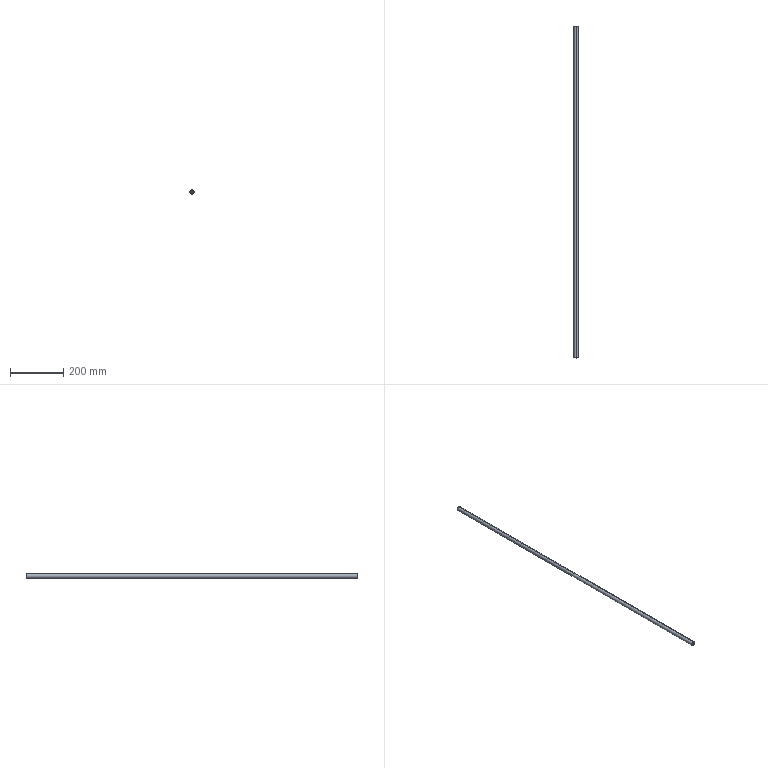Part | STEP file | PN_0027 | 1 solid | 16 faces | box 16 x 1252 x 16 mm | volume 251030 mm3 | cone 8 | cylinder 6 | plane 2 | commonest cylinder face diameters 5 x4 16 x2
STEP:
#1=CARTESIAN_POINT('',(0.,0.,0.));
#2=DIRECTION('',(0.,0.,1.));
#3=DIRECTION('',(1.,0.,0.));
#4=AXIS2_PLACEMENT_3D('',#1,#2,#3);
#5=CARTESIAN_POINT('',(0.,1252.,7.5));
#6=VERTEX_POINT('',#5);
#7=CARTESIAN_POINT('',(0.,1252.,-7.5));
#8=VERTEX_POINT('',#7);
#9=CARTESIAN_POINT('',(0.,1252.,0.));
#10=DIRECTION('',(0.,1.,0.));
#11=DIRECTION('',(0.,0.,1.));
#12=AXIS2_PLACEMENT_3D('',#9,#10,#11);
#13=CIRCLE('',#12,7.5);
#14=CARTESIAN_POINT('',(0.,1252.,0.));
#15=DIRECTION('',(0.,-1.,0.));
#16=DIRECTION('',(0.,0.,-1.));
#17=AXIS2_PLACEMENT_3D('',#14,#15,#16);
#18=CONICAL_SURFACE('',#17,7.5,0.7854);
#19=CARTESIAN_POINT('',(3.142,0.));
#20=DIRECTION('',(-1.,0.));
#21=VECTOR('',#20,1.);
#22=LINE('',#19,#21);
#23=(GEOMETRIC_REPRESENTATION_CONTEXT(2)PARAMETRIC_REPRESENTATION_CONTEXT()REPRESENTATION_CONTEXT('',''));
#24=DEFINITIONAL_REPRESENTATION('',(#22),#23);
#25=PCURVE('',#18,#24);
#26=CARTESIAN_POINT('',(0.,1252.,0.));
#27=DIRECTION('',(0.,1.,0.));
#28=DIRECTION('',(0.,0.,1.));
#29=AXIS2_PLACEMENT_3D('',#26,#27,#28);
#30=PLANE('',#29);
#31=CARTESIAN_POINT('',(0.,0.));
#32=DIRECTION('',(1.,0.));
#33=AXIS2_PLACEMENT_2D('',#31,#32);
#34=CIRCLE('',#33,7.5);
#35=(GEOMETRIC_REPRESENTATION_CONTEXT(2)PARAMETRIC_REPRESENTATION_CONTEXT()REPRESENTATION_CONTEXT('',''));
#36=DEFINITIONAL_REPRESENTATION('',(#34),#35);
#37=PCURVE('',#30,#36);
#38=SURFACE_CURVE('',#13,(#25,#37),.PCURVE_S1.);
#39=EDGE_CURVE('',#6,#8,#38,.T.);
#40=ORIENTED_EDGE('',*,*,#39,.F.);
#41=CARTESIAN_POINT('',(0.,1251.5,8.));
#42=VERTEX_POINT('',#41);
#43=CARTESIAN_POINT('',(0.,1252.,7.5));
#44=DIRECTION('',(0.,-0.7071,0.7071));
#45=VECTOR('',#44,1.);
#46=LINE('',#43,#45);
#47=CARTESIAN_POINT('',(3.142,0.));
#48=DIRECTION('',(0.,1.));
#49=VECTOR('',#48,1.);
#50=LINE('',#47,#49);
#51=(GEOMETRIC_REPRESENTATION_CONTEXT(2)PARAMETRIC_REPRESENTATION_CONTEXT()REPRESENTATION_CONTEXT('',''));
#52=DEFINITIONAL_REPRESENTATION('',(#50),#51);
#53=PCURVE('',#18,#52);
#54=CARTESIAN_POINT('',(0.,1252.,0.));
#55=DIRECTION('',(0.,-1.,0.));
#56=DIRECTION('',(0.,0.,-1.));
#57=AXIS2_PLACEMENT_3D('',#54,#55,#56);
#58=CONICAL_SURFACE('',#57,7.5,0.7854);
#59=CARTESIAN_POINT('',(3.142,0.));
#60=DIRECTION('',(0.,1.));
#61=VECTOR('',#60,1.);
#62=LINE('',#59,#61);
#63=(GEOMETRIC_REPRESENTATION_CONTEXT(2)PARAMETRIC_REPRESENTATION_CONTEXT()REPRESENTATION_CONTEXT('',''));
#64=DEFINITIONAL_REPRESENTATION('',(#62),#63);
#65=PCURVE('',#58,#64);
#66=SURFACE_CURVE('',#46,(#53,#65),.PCURVE_S1.);
#67=EDGE_CURVE('',#6,#42,#66,.T.);
#68=ORIENTED_EDGE('',*,*,#67,.T.);
#69=CARTESIAN_POINT('',(0.,1251.5,-8.));
#70=VERTEX_POINT('',#69);
#71=CARTESIAN_POINT('',(0.,1251.5,0.));
#72=DIRECTION('',(0.,-1.,0.));
#73=DIRECTION('',(0.,0.,1.));
#74=AXIS2_PLACEMENT_3D('',#71,#72,#73);
#75=CIRCLE('',#74,8.);
#76=CARTESIAN_POINT('',(-3.142,0.5));
#77=DIRECTION('',(1.,0.));
#78=VECTOR('',#77,1.);
#79=LINE('',#76,#78);
#80=(GEOMETRIC_REPRESENTATION_CONTEXT(2)PARAMETRIC_REPRESENTATION_CONTEXT()REPRESENTATION_CONTEXT('',''));
#81=DEFINITIONAL_REPRESENTATION('',(#79),#80);
#82=PCURVE('',#18,#81);
#83=CARTESIAN_POINT('',(0.,1252.,0.));
#84=DIRECTION('',(0.,-1.,0.));
#85=DIRECTION('',(0.,0.,-1.));
#86=AXIS2_PLACEMENT_3D('',#83,#84,#85);
#87=CYLINDRICAL_SURFACE('',#86,8.);
#88=CARTESIAN_POINT('',(-3.142,0.5));
#89=DIRECTION('',(1.,0.));
#90=VECTOR('',#89,1.);
#91=LINE('',#88,#90);
#92=(GEOMETRIC_REPRESENTATION_CONTEXT(2)PARAMETRIC_REPRESENTATION_CONTEXT()REPRESENTATION_CONTEXT('',''));
#93=DEFINITIONAL_REPRESENTATION('',(#91),#92);
#94=PCURVE('',#87,#93);
#95=SURFACE_CURVE('',#75,(#82,#94),.PCURVE_S1.);
#96=EDGE_CURVE('',#70,#42,#95,.T.);
#97=ORIENTED_EDGE('',*,*,#96,.F.);
#98=CARTESIAN_POINT('',(0.,1252.,-7.5));
#99=DIRECTION('',(0.,-0.7071,-0.7071));
#100=VECTOR('',#99,1.);
#101=LINE('',#98,#100);
#102=CARTESIAN_POINT('',(0.,0.));
#103=DIRECTION('',(0.,1.));
#104=VECTOR('',#103,1.);
#105=LINE('',#102,#104);
#106=(GEOMETRIC_REPRESENTATION_CONTEXT(2)PARAMETRIC_REPRESENTATION_CONTEXT()REPRESENTATION_CONTEXT('',''));
#107=DEFINITIONAL_REPRESENTATION('',(#105),#106);
#108=PCURVE('',#18,#107);
#109=CARTESIAN_POINT('',(6.283,0.));
#110=DIRECTION('',(0.,1.));
#111=VECTOR('',#110,1.);
#112=LINE('',#109,#111);
#113=(GEOMETRIC_REPRESENTATION_CONTEXT(2)PARAMETRIC_REPRESENTATION_CONTEXT()REPRESENTATION_CONTEXT('',''));
#114=DEFINITIONAL_REPRESENTATION('',(#112),#113);
#115=PCURVE('',#58,#114);
#116=SURFACE_CURVE('',#101,(#108,#115),.PCURVE_S1.);
#117=EDGE_CURVE('',#8,#70,#116,.T.);
#118=ORIENTED_EDGE('',*,*,#117,.F.);
#119=EDGE_LOOP('',(#40,#68,#97,#118));
#120=FACE_BOUND('',#119,.T.);
#121=ADVANCED_FACE('',(#120),#18,.T.);
#122=CARTESIAN_POINT('',(0.,0.,-7.5));
#123=VERTEX_POINT('',#122);
#124=CARTESIAN_POINT('',(0.,0.,7.5));
#125=VERTEX_POINT('',#124);
#126=CARTESIAN_POINT('',(0.,0.,0.));
#127=DIRECTION('',(0.,-1.,0.));
#128=DIRECTION('',(0.,0.,1.));
#129=AXIS2_PLACEMENT_3D('',#126,#127,#128);
#130=CIRCLE('',#129,7.5);
#131=CARTESIAN_POINT('',(0.,0.5,0.));
#132=DIRECTION('',(0.,1.,0.));
#133=DIRECTION('',(0.,0.,1.));
#134=AXIS2_PLACEMENT_3D('',#131,#132,#133);
#135=CONICAL_SURFACE('',#134,8.,0.7854);
#136=CARTESIAN_POINT('',(6.283,-0.5));
#137=DIRECTION('',(-1.,0.));
#138=VECTOR('',#137,1.);
#139=LINE('',#136,#138);
#140=(GEOMETRIC_REPRESENTATION_CONTEXT(2)PARAMETRIC_REPRESENTATION_CONTEXT()REPRESENTATION_CONTEXT('',''));
#141=DEFINITIONAL_REPRESENTATION('',(#139),#140);
#142=PCURVE('',#135,#141);
#143=CARTESIAN_POINT('',(0.,0.,0.));
#144=DIRECTION('',(0.,1.,0.));
#145=DIRECTION('',(0.,0.,1.));
#146=AXIS2_PLACEMENT_3D('',#143,#144,#145);
#147=PLANE('',#146);
#148=CARTESIAN_POINT('',(7.5,0.));
#149=CARTESIAN_POINT('',(7.5,-12.99));
#150=CARTESIAN_POINT('',(-3.75,-6.495));
#151=CARTESIAN_POINT('',(-15.,0.));
#152=CARTESIAN_POINT('',(-3.75,6.495));
#153=CARTESIAN_POINT('',(7.5,12.99));
#154=CARTESIAN_POINT('',(7.5,0.));
#155=(BOUNDED_CURVE()B_SPLINE_CURVE(2,(#148,#149,#150,#151,#152,#153,#154),.UNSPECIFIED.,.T.,.F.)B_SPLINE_CURVE_WITH_KNOTS((1,2,2,2,2,1),(-2.094,0.,2.094,4.189,6.283,8.378),.UNSPECIFIED.)CURVE()GEOMETRIC_REPRESENTATION_ITEM()RATIONAL_B_SPLINE_CURVE((1.,0.5,1.,0.5,1.,0.5,1.))REPRESENTATION_ITEM(''));
#156=(GEOMETRIC_REPRESENTATION_CONTEXT(2)PARAMETRIC_REPRESENTATION_CONTEXT()REPRESENTATION_CONTEXT('',''));
#157=DEFINITIONAL_REPRESENTATION('',(#155),#156);
#158=PCURVE('',#147,#157);
#159=SURFACE_CURVE('',#130,(#142,#158),.PCURVE_S1.);
#160=EDGE_CURVE('',#123,#125,#159,.T.);
#161=ORIENTED_EDGE('',*,*,#160,.F.);
#162=CARTESIAN_POINT('',(0.,0.5,-8.));
#163=VERTEX_POINT('',#162);
#164=CARTESIAN_POINT('',(0.,0.5,-8.));
#165=DIRECTION('',(0.,0.7071,-0.7071));
#166=VECTOR('',#165,1.);
#167=LINE('',#164,#166);
#168=CARTESIAN_POINT('',(3.142,0.));
#169=DIRECTION('',(0.,1.));
#170=VECTOR('',#169,1.);
#171=LINE('',#168,#170);
#172=(GEOMETRIC_REPRESENTATION_CONTEXT(2)PARAMETRIC_REPRESENTATION_CONTEXT()REPRESENTATION_CONTEXT('',''));
#173=DEFINITIONAL_REPRESENTATION('',(#171),#172);
#174=PCURVE('',#135,#173);
#175=CARTESIAN_POINT('',(0.,0.5,0.));
#176=DIRECTION('',(0.,1.,0.));
#177=DIRECTION('',(0.,0.,1.));
#178=AXIS2_PLACEMENT_3D('',#175,#176,#177);
#179=CONICAL_SURFACE('',#178,8.,0.7854);
#180=CARTESIAN_POINT('',(3.142,0.));
#181=DIRECTION('',(0.,1.));
#182=VECTOR('',#181,1.);
#183=LINE('',#180,#182);
#184=(GEOMETRIC_REPRESENTATION_CONTEXT(2)PARAMETRIC_REPRESENTATION_CONTEXT()REPRESENTATION_CONTEXT('',''));
#185=DEFINITIONAL_REPRESENTATION('',(#183),#184);
#186=PCURVE('',#179,#185);
#187=SURFACE_CURVE('',#167,(#174,#186),.PCURVE_S1.);
#188=EDGE_CURVE('',#123,#163,#187,.T.);
#189=ORIENTED_EDGE('',*,*,#188,.T.);
#190=CARTESIAN_POINT('',(0.,0.5,8.));
#191=VERTEX_POINT('',#190);
#192=CARTESIAN_POINT('',(0.,0.5,0.));
#193=DIRECTION('',(0.,1.,0.));
#194=DIRECTION('',(0.,0.,1.));
#195=AXIS2_PLACEMENT_3D('',#192,#193,#194);
#196=CIRCLE('',#195,8.);
#197=CARTESIAN_POINT('',(0.,0.));
#198=DIRECTION('',(1.,0.));
#199=VECTOR('',#198,1.);
#200=LINE('',#197,#199);
#201=(GEOMETRIC_REPRESENTATION_CONTEXT(2)PARAMETRIC_REPRESENTATION_CONTEXT()REPRESENTATION_CONTEXT('',''));
#202=DEFINITIONAL_REPRESENTATION('',(#200),#201);
#203=PCURVE('',#135,#202);
#204=CARTESIAN_POINT('',(3.142,1251.5));
#205=DIRECTION('',(-1.,0.));
#206=VECTOR('',#205,1.);
#207=LINE('',#204,#206);
#208=(GEOMETRIC_REPRESENTATION_CONTEXT(2)PARAMETRIC_REPRESENTATION_CONTEXT()REPRESENTATION_CONTEXT('',''));
#209=DEFINITIONAL_REPRESENTATION('',(#207),#208);
#210=PCURVE('',#87,#209);
#211=SURFACE_CURVE('',#196,(#203,#210),.PCURVE_S1.);
#212=EDGE_CURVE('',#191,#163,#211,.T.);
#213=ORIENTED_EDGE('',*,*,#212,.F.);
#214=CARTESIAN_POINT('',(0.,0.5,8.));
#215=DIRECTION('',(0.,0.7071,0.7071));
#216=VECTOR('',#215,1.);
#217=LINE('',#214,#216);
#218=CARTESIAN_POINT('',(0.,0.));
#219=DIRECTION('',(0.,1.));
#220=VECTOR('',#219,1.);
#221=LINE('',#218,#220);
#222=(GEOMETRIC_REPRESENTATION_CONTEXT(2)PARAMETRIC_REPRESENTATION_CONTEXT()REPRESENTATION_CONTEXT('',''));
#223=DEFINITIONAL_REPRESENTATION('',(#221),#222);
#224=PCURVE('',#135,#223);
#225=CARTESIAN_POINT('',(6.283,0.));
#226=DIRECTION('',(0.,1.));
#227=VECTOR('',#226,1.);
#228=LINE('',#225,#227);
#229=(GEOMETRIC_REPRESENTATION_CONTEXT(2)PARAMETRIC_REPRESENTATION_CONTEXT()REPRESENTATION_CONTEXT('',''));
#230=DEFINITIONAL_REPRESENTATION('',(#228),#229);
#231=PCURVE('',#179,#230);
#232=SURFACE_CURVE('',#217,(#224,#231),.PCURVE_S1.);
#233=EDGE_CURVE('',#125,#191,#232,.T.);
#234=ORIENTED_EDGE('',*,*,#233,.F.);
#235=EDGE_LOOP('',(#161,#189,#213,#234));
#236=FACE_BOUND('',#235,.T.);
#237=ADVANCED_FACE('',(#236),#135,.T.);
#238=CARTESIAN_POINT('',(0.,17.,-2.5));
#239=VERTEX_POINT('',#238);
#240=CARTESIAN_POINT('',(0.,0.,-2.5));
#241=VERTEX_POINT('',#240);
#242=CARTESIAN_POINT('',(0.,0.,-2.5));
#243=DIRECTION('',(0.,-1.,0.));
#244=VECTOR('',#243,1.);
#245=LINE('',#242,#244);
#246=CARTESIAN_POINT('',(0.,0.,0.));
#247=DIRECTION('',(0.,-1.,0.));
#248=DIRECTION('',(0.,0.,-1.));
#249=AXIS2_PLACEMENT_3D('',#246,#247,#248);
#250=CYLINDRICAL_SURFACE('',#249,2.5);
#251=CARTESIAN_POINT('',(6.283,0.));
#252=DIRECTION('',(0.,1.));
#253=VECTOR('',#252,1.);
#254=LINE('',#251,#253);
#255=(GEOMETRIC_REPRESENTATION_CONTEXT(2)PARAMETRIC_REPRESENTATION_CONTEXT()REPRESENTATION_CONTEXT('',''));
#256=DEFINITIONAL_REPRESENTATION('',(#254),#255);
#257=PCURVE('',#250,#256);
#258=CARTESIAN_POINT('',(0.,0.,0.));
#259=DIRECTION('',(0.,-1.,0.));
#260=DIRECTION('',(0.,0.,-1.));
#261=AXIS2_PLACEMENT_3D('',#258,#259,#260);
#262=CYLINDRICAL_SURFACE('',#261,2.5);
#263=CARTESIAN_POINT('',(0.,0.));
#264=DIRECTION('',(0.,1.));
#265=VECTOR('',#264,1.);
#266=LINE('',#263,#265);
#267=(GEOMETRIC_REPRESENTATION_CONTEXT(2)PARAMETRIC_REPRESENTATION_CONTEXT()REPRESENTATION_CONTEXT('',''));
#268=DEFINITIONAL_REPRESENTATION('',(#266),#267);
#269=PCURVE('',#262,#268);
#270=SURFACE_CURVE('',#245,(#257,#269),.PCURVE_S1.);
#271=EDGE_CURVE('',#239,#241,#270,.T.);
#272=ORIENTED_EDGE('',*,*,#271,.T.);
#273=CARTESIAN_POINT('',(0.,0.,2.5));
#274=VERTEX_POINT('',#273);
#275=CARTESIAN_POINT('',(0.,0.,0.));
#276=DIRECTION('',(0.,-1.,0.));
#277=DIRECTION('',(0.,0.,-1.));
#278=AXIS2_PLACEMENT_3D('',#275,#276,#277);
#279=CIRCLE('',#278,2.5);
#280=CARTESIAN_POINT('',(0.,0.));
#281=DIRECTION('',(1.,0.));
#282=VECTOR('',#281,1.);
#283=LINE('',#280,#282);
#284=(GEOMETRIC_REPRESENTATION_CONTEXT(2)PARAMETRIC_REPRESENTATION_CONTEXT()REPRESENTATION_CONTEXT('',''));
#285=DEFINITIONAL_REPRESENTATION('',(#283),#284);
#286=PCURVE('',#250,#285);
#287=CARTESIAN_POINT('',(-2.5,0.));
#288=CARTESIAN_POINT('',(-2.5,4.33));
#289=CARTESIAN_POINT('',(1.25,2.165));
#290=CARTESIAN_POINT('',(5.,0.));
#291=CARTESIAN_POINT('',(1.25,-2.165));
#292=CARTESIAN_POINT('',(-2.5,-4.33));
#293=CARTESIAN_POINT('',(-2.5,0.));
#294=(BOUNDED_CURVE()B_SPLINE_CURVE(2,(#287,#288,#289,#290,#291,#292,#293),.UNSPECIFIED.,.T.,.F.)B_SPLINE_CURVE_WITH_KNOTS((1,2,2,2,2,1),(-2.094,0.,2.094,4.189,6.283,8.378),.UNSPECIFIED.)CURVE()GEOMETRIC_REPRESENTATION_ITEM()RATIONAL_B_SPLINE_CURVE((1.,0.5,1.,0.5,1.,0.5,1.))REPRESENTATION_ITEM(''));
#295=(GEOMETRIC_REPRESENTATION_CONTEXT(2)PARAMETRIC_REPRESENTATION_CONTEXT()REPRESENTATION_CONTEXT('',''));
#296=DEFINITIONAL_REPRESENTATION('',(#294),#295);
#297=PCURVE('',#147,#296);
#298=SURFACE_CURVE('',#279,(#286,#297),.PCURVE_S1.);
#299=EDGE_CURVE('',#274,#241,#298,.T.);
#300=ORIENTED_EDGE('',*,*,#299,.F.);
#301=CARTESIAN_POINT('',(0.,17.,2.5));
#302=VERTEX_POINT('',#301);
#303=CARTESIAN_POINT('',(0.,0.,2.5));
#304=DIRECTION('',(0.,-1.,0.));
#305=VECTOR('',#304,1.);
#306=LINE('',#303,#305);
#307=CARTESIAN_POINT('',(3.142,0.));
#308=DIRECTION('',(0.,1.));
#309=VECTOR('',#308,1.);
#310=LINE('',#307,#309);
#311=(GEOMETRIC_REPRESENTATION_CONTEXT(2)PARAMETRIC_REPRESENTATION_CONTEXT()REPRESENTATION_CONTEXT('',''));
#312=DEFINITIONAL_REPRESENTATION('',(#310),#311);
#313=PCURVE('',#250,#312);
#314=CARTESIAN_POINT('',(3.142,0.));
#315=DIRECTION('',(0.,1.));
#316=VECTOR('',#315,1.);
#317=LINE('',#314,#316);
#318=(GEOMETRIC_REPRESENTATION_CONTEXT(2)PARAMETRIC_REPRESENTATION_CONTEXT()REPRESENTATION_CONTEXT('',''));
#319=DEFINITIONAL_REPRESENTATION('',(#317),#318);
#320=PCURVE('',#262,#319);
#321=SURFACE_CURVE('',#306,(#313,#320),.PCURVE_S1.);
#322=EDGE_CURVE('',#302,#274,#321,.T.);
#323=ORIENTED_EDGE('',*,*,#322,.F.);
#324=CARTESIAN_POINT('',(0.,17.,0.));
#325=DIRECTION('',(0.,-1.,0.));
#326=DIRECTION('',(0.,0.,-1.));
#327=AXIS2_PLACEMENT_3D('',#324,#325,#326);
#328=CIRCLE('',#327,2.5);
#329=CARTESIAN_POINT('',(0.,-17.));
#330=DIRECTION('',(1.,0.));
#331=VECTOR('',#330,1.);
#332=LINE('',#329,#331);
#333=(GEOMETRIC_REPRESENTATION_CONTEXT(2)PARAMETRIC_REPRESENTATION_CONTEXT()REPRESENTATION_CONTEXT('',''));
#334=DEFINITIONAL_REPRESENTATION('',(#332),#333);
#335=PCURVE('',#250,#334);
#336=CARTESIAN_POINT('',(0.,17.,0.));
#337=DIRECTION('',(0.,-1.,0.));
#338=DIRECTION('',(0.,0.,-1.));
#339=AXIS2_PLACEMENT_3D('',#336,#337,#338);
#340=CONICAL_SURFACE('',#339,2.5,1.03);
#341=CARTESIAN_POINT('',(0.,0.));
#342=DIRECTION('',(1.,0.));
#343=VECTOR('',#342,1.);
#344=LINE('',#341,#343);
#345=(GEOMETRIC_REPRESENTATION_CONTEXT(2)PARAMETRIC_REPRESENTATION_CONTEXT()REPRESENTATION_CONTEXT('',''));
#346=DEFINITIONAL_REPRESENTATION('',(#344),#345);
#347=PCURVE('',#340,#346);
#348=SURFACE_CURVE('',#328,(#335,#347),.PCURVE_S1.);
#349=EDGE_CURVE('',#302,#239,#348,.T.);
#350=ORIENTED_EDGE('',*,*,#349,.T.);
#351=EDGE_LOOP('',(#272,#300,#323,#350));
#352=FACE_BOUND('',#351,.F.);
#353=ADVANCED_FACE('',(#352),#250,.F.);
#354=ORIENTED_EDGE('',*,*,#349,.F.);
#355=CARTESIAN_POINT('',(0.,18.502,0.));
#356=VERTEX_POINT('',#355);
#357=CARTESIAN_POINT('',(0.,17.,2.5));
#358=DIRECTION('',(0.,-0.515,0.8572));
#359=VECTOR('',#358,1.);
#360=LINE('',#357,#359);
#361=CARTESIAN_POINT('',(3.142,0.));
#362=DIRECTION('',(0.,1.));
#363=VECTOR('',#362,1.);
#364=LINE('',#361,#363);
#365=(GEOMETRIC_REPRESENTATION_CONTEXT(2)PARAMETRIC_REPRESENTATION_CONTEXT()REPRESENTATION_CONTEXT('',''));
#366=DEFINITIONAL_REPRESENTATION('',(#364),#365);
#367=PCURVE('',#340,#366);
#368=CARTESIAN_POINT('',(0.,17.,0.));
#369=DIRECTION('',(0.,-1.,0.));
#370=DIRECTION('',(0.,0.,-1.));
#371=AXIS2_PLACEMENT_3D('',#368,#369,#370);
#372=CONICAL_SURFACE('',#371,2.5,1.03);
#373=CARTESIAN_POINT('',(3.142,0.));
#374=DIRECTION('',(0.,1.));
#375=VECTOR('',#374,1.);
#376=LINE('',#373,#375);
#377=(GEOMETRIC_REPRESENTATION_CONTEXT(2)PARAMETRIC_REPRESENTATION_CONTEXT()REPRESENTATION_CONTEXT('',''));
#378=DEFINITIONAL_REPRESENTATION('',(#376),#377);
#379=PCURVE('',#372,#378);
#380=SURFACE_CURVE('',#360,(#367,#379),.PCURVE_S1.);
#381=EDGE_CURVE('',#356,#302,#380,.T.);
#382=ORIENTED_EDGE('',*,*,#381,.F.);
#383=CARTESIAN_POINT('',(0.,17.,-2.5));
#384=DIRECTION('',(0.,-0.515,-0.8572));
#385=VECTOR('',#384,1.);
#386=LINE('',#383,#385);
#387=CARTESIAN_POINT('',(6.283,0.));
#388=DIRECTION('',(0.,1.));
#389=VECTOR('',#388,1.);
#390=LINE('',#387,#389);
#391=(GEOMETRIC_REPRESENTATION_CONTEXT(2)PARAMETRIC_REPRESENTATION_CONTEXT()REPRESENTATION_CONTEXT('',''));
#392=DEFINITIONAL_REPRESENTATION('',(#390),#391);
#393=PCURVE('',#340,#392);
#394=CARTESIAN_POINT('',(0.,0.));
#395=DIRECTION('',(0.,1.));
#396=VECTOR('',#395,1.);
#397=LINE('',#394,#396);
#398=(GEOMETRIC_REPRESENTATION_CONTEXT(2)PARAMETRIC_REPRESENTATION_CONTEXT()REPRESENTATION_CONTEXT('',''));
#399=DEFINITIONAL_REPRESENTATION('',(#397),#398);
#400=PCURVE('',#372,#399);
#401=SURFACE_CURVE('',#386,(#393,#400),.PCURVE_S1.);
#402=EDGE_CURVE('',#356,#239,#401,.T.);
#403=ORIENTED_EDGE('',*,*,#402,.T.);
#404=EDGE_LOOP('',(#354,#382,#403));
#405=FACE_BOUND('',#404,.F.);
#406=ADVANCED_FACE('',(#405),#340,.F.);
#407=CARTESIAN_POINT('',(0.,1235.,2.5));
#408=VERTEX_POINT('',#407);
#409=CARTESIAN_POINT('',(0.,1252.,2.5));
#410=VERTEX_POINT('',#409);
#411=CARTESIAN_POINT('',(0.,1252.,2.5));
#412=DIRECTION('',(0.,1.,0.));
#413=VECTOR('',#412,1.);
#414=LINE('',#411,#413);
#415=CARTESIAN_POINT('',(0.,1252.,0.));
#416=DIRECTION('',(0.,1.,0.));
#417=DIRECTION('',(0.,0.,1.));
#418=AXIS2_PLACEMENT_3D('',#415,#416,#417);
#419=CYLINDRICAL_SURFACE('',#418,2.5);
#420=CARTESIAN_POINT('',(6.283,0.));
#421=DIRECTION('',(0.,1.));
#422=VECTOR('',#421,1.);
#423=LINE('',#420,#422);
#424=(GEOMETRIC_REPRESENTATION_CONTEXT(2)PARAMETRIC_REPRESENTATION_CONTEXT()REPRESENTATION_CONTEXT('',''));
#425=DEFINITIONAL_REPRESENTATION('',(#423),#424);
#426=PCURVE('',#419,#425);
#427=CARTESIAN_POINT('',(0.,1252.,0.));
#428=DIRECTION('',(0.,1.,0.));
#429=DIRECTION('',(0.,0.,1.));
#430=AXIS2_PLACEMENT_3D('',#427,#428,#429);
#431=CYLINDRICAL_SURFACE('',#430,2.5);
#432=CARTESIAN_POINT('',(0.,0.));
#433=DIRECTION('',(0.,1.));
#434=VECTOR('',#433,1.);
#435=LINE('',#432,#434);
#436=(GEOMETRIC_REPRESENTATION_CONTEXT(2)PARAMETRIC_REPRESENTATION_CONTEXT()REPRESENTATION_CONTEXT('',''));
#437=DEFINITIONAL_REPRESENTATION('',(#435),#436);
#438=PCURVE('',#431,#437);
#439=SURFACE_CURVE('',#414,(#426,#438),.PCURVE_S1.);
#440=EDGE_CURVE('',#408,#410,#439,.T.);
#441=ORIENTED_EDGE('',*,*,#440,.T.);
#442=CARTESIAN_POINT('',(0.,1252.,-2.5));
#443=VERTEX_POINT('',#442);
#444=CARTESIAN_POINT('',(0.,1252.,0.));
#445=DIRECTION('',(0.,1.,0.));
#446=DIRECTION('',(0.,0.,1.));
#447=AXIS2_PLACEMENT_3D('',#444,#445,#446);
#448=CIRCLE('',#447,2.5);
#449=CARTESIAN_POINT('',(0.,0.));
#450=DIRECTION('',(1.,0.));
#451=VECTOR('',#450,1.);
#452=LINE('',#449,#451);
#453=(GEOMETRIC_REPRESENTATION_CONTEXT(2)PARAMETRIC_REPRESENTATION_CONTEXT()REPRESENTATION_CONTEXT('',''));
#454=DEFINITIONAL_REPRESENTATION('',(#452),#453);
#455=PCURVE('',#419,#454);
#456=CARTESIAN_POINT('',(0.,0.));
#457=DIRECTION('',(1.,0.));
#458=AXIS2_PLACEMENT_2D('',#456,#457);
#459=CIRCLE('',#458,2.5);
#460=(GEOMETRIC_REPRESENTATION_CONTEXT(2)PARAMETRIC_REPRESENTATION_CONTEXT()REPRESENTATION_CONTEXT('',''));
#461=DEFINITIONAL_REPRESENTATION('',(#459),#460);
#462=PCURVE('',#30,#461);
#463=SURFACE_CURVE('',#448,(#455,#462),.PCURVE_S1.);
#464=EDGE_CURVE('',#443,#410,#463,.T.);
#465=ORIENTED_EDGE('',*,*,#464,.F.);
#466=CARTESIAN_POINT('',(0.,1235.,-2.5));
#467=VERTEX_POINT('',#466);
#468=CARTESIAN_POINT('',(0.,1252.,-2.5));
#469=DIRECTION('',(0.,1.,0.));
#470=VECTOR('',#469,1.);
#471=LINE('',#468,#470);
#472=CARTESIAN_POINT('',(3.142,0.));
#473=DIRECTION('',(0.,1.));
#474=VECTOR('',#473,1.);
#475=LINE('',#472,#474);
#476=(GEOMETRIC_REPRESENTATION_CONTEXT(2)PARAMETRIC_REPRESENTATION_CONTEXT()REPRESENTATION_CONTEXT('',''));
#477=DEFINITIONAL_REPRESENTATION('',(#475),#476);
#478=PCURVE('',#419,#477);
#479=CARTESIAN_POINT('',(3.142,0.));
#480=DIRECTION('',(0.,1.));
#481=VECTOR('',#480,1.);
#482=LINE('',#479,#481);
#483=(GEOMETRIC_REPRESENTATION_CONTEXT(2)PARAMETRIC_REPRESENTATION_CONTEXT()REPRESENTATION_CONTEXT('',''));
#484=DEFINITIONAL_REPRESENTATION('',(#482),#483);
#485=PCURVE('',#431,#484);
#486=SURFACE_CURVE('',#471,(#478,#485),.PCURVE_S1.);
#487=EDGE_CURVE('',#467,#443,#486,.T.);
#488=ORIENTED_EDGE('',*,*,#487,.F.);
#489=CARTESIAN_POINT('',(0.,1235.,0.));
#490=DIRECTION('',(0.,1.,0.));
#491=DIRECTION('',(0.,0.,1.));
#492=AXIS2_PLACEMENT_3D('',#489,#490,#491);
#493=CIRCLE('',#492,2.5);
#494=CARTESIAN_POINT('',(0.,-17.));
#495=DIRECTION('',(1.,0.));
#496=VECTOR('',#495,1.);
#497=LINE('',#494,#496);
#498=(GEOMETRIC_REPRESENTATION_CONTEXT(2)PARAMETRIC_REPRESENTATION_CONTEXT()REPRESENTATION_CONTEXT('',''));
#499=DEFINITIONAL_REPRESENTATION('',(#497),#498);
#500=PCURVE('',#419,#499);
#501=CARTESIAN_POINT('',(0.,1235.,0.));
#502=DIRECTION('',(0.,1.,0.));
#503=DIRECTION('',(0.,0.,1.));
#504=AXIS2_PLACEMENT_3D('',#501,#502,#503);
#505=CONICAL_SURFACE('',#504,2.5,1.03);
#506=CARTESIAN_POINT('',(0.,0.));
#507=DIRECTION('',(1.,0.));
#508=VECTOR('',#507,1.);
#509=LINE('',#506,#508);
#510=(GEOMETRIC_REPRESENTATION_CONTEXT(2)PARAMETRIC_REPRESENTATION_CONTEXT()REPRESENTATION_CONTEXT('',''));
#511=DEFINITIONAL_REPRESENTATION('',(#509),#510);
#512=PCURVE('',#505,#511);
#513=SURFACE_CURVE('',#493,(#500,#512),.PCURVE_S1.);
#514=EDGE_CURVE('',#467,#408,#513,.T.);
#515=ORIENTED_EDGE('',*,*,#514,.T.);
#516=EDGE_LOOP('',(#441,#465,#488,#515));
#517=FACE_BOUND('',#516,.F.);
#518=ADVANCED_FACE('',(#517),#419,.F.);
#519=ORIENTED_EDGE('',*,*,#514,.F.);
#520=CARTESIAN_POINT('',(0.,1233.498,0.));
#521=VERTEX_POINT('',#520);
#522=CARTESIAN_POINT('',(0.,1235.,-2.5));
#523=DIRECTION('',(0.,0.515,-0.8572));
#524=VECTOR('',#523,1.);
#525=LINE('',#522,#524);
#526=CARTESIAN_POINT('',(3.142,0.));
#527=DIRECTION('',(0.,1.));
#528=VECTOR('',#527,1.);
#529=LINE('',#526,#528);
#530=(GEOMETRIC_REPRESENTATION_CONTEXT(2)PARAMETRIC_REPRESENTATION_CONTEXT()REPRESENTATION_CONTEXT('',''));
#531=DEFINITIONAL_REPRESENTATION('',(#529),#530);
#532=PCURVE('',#505,#531);
#533=CARTESIAN_POINT('',(0.,1235.,0.));
#534=DIRECTION('',(0.,1.,0.));
#535=DIRECTION('',(0.,0.,1.));
#536=AXIS2_PLACEMENT_3D('',#533,#534,#535);
#537=CONICAL_SURFACE('',#536,2.5,1.03);
#538=CARTESIAN_POINT('',(3.142,0.));
#539=DIRECTION('',(0.,1.));
#540=VECTOR('',#539,1.);
#541=LINE('',#538,#540);
#542=(GEOMETRIC_REPRESENTATION_CONTEXT(2)PARAMETRIC_REPRESENTATION_CONTEXT()REPRESENTATION_CONTEXT('',''));
#543=DEFINITIONAL_REPRESENTATION('',(#541),#542);
#544=PCURVE('',#537,#543);
#545=SURFACE_CURVE('',#525,(#532,#544),.PCURVE_S1.);
#546=EDGE_CURVE('',#521,#467,#545,.T.);
#547=ORIENTED_EDGE('',*,*,#546,.F.);
#548=CARTESIAN_POINT('',(0.,1235.,2.5));
#549=DIRECTION('',(0.,0.515,0.8572));
#550=VECTOR('',#549,1.);
#551=LINE('',#548,#550);
#552=CARTESIAN_POINT('',(6.283,0.));
#553=DIRECTION('',(0.,1.));
#554=VECTOR('',#553,1.);
#555=LINE('',#552,#554);
#556=(GEOMETRIC_REPRESENTATION_CONTEXT(2)PARAMETRIC_REPRESENTATION_CONTEXT()REPRESENTATION_CONTEXT('',''));
#557=DEFINITIONAL_REPRESENTATION('',(#555),#556);
#558=PCURVE('',#505,#557);
#559=CARTESIAN_POINT('',(0.,0.));
#560=DIRECTION('',(0.,1.));
#561=VECTOR('',#560,1.);
#562=LINE('',#559,#561);
#563=(GEOMETRIC_REPRESENTATION_CONTEXT(2)PARAMETRIC_REPRESENTATION_CONTEXT()REPRESENTATION_CONTEXT('',''));
#564=DEFINITIONAL_REPRESENTATION('',(#562),#563);
#565=PCURVE('',#537,#564);
#566=SURFACE_CURVE('',#551,(#558,#565),.PCURVE_S1.);
#567=EDGE_CURVE('',#521,#408,#566,.T.);
#568=ORIENTED_EDGE('',*,*,#567,.T.);
#569=EDGE_LOOP('',(#519,#547,#568));
#570=FACE_BOUND('',#569,.F.);
#571=ADVANCED_FACE('',(#570),#505,.F.);
#572=ORIENTED_EDGE('',*,*,#96,.T.);
#573=CARTESIAN_POINT('',(0.,1252.,8.));
#574=DIRECTION('',(0.,-1.,0.));
#575=VECTOR('',#574,1.);
#576=LINE('',#573,#575);
#577=CARTESIAN_POINT('',(3.142,0.));
#578=DIRECTION('',(0.,1.));
#579=VECTOR('',#578,1.);
#580=LINE('',#577,#579);
#581=(GEOMETRIC_REPRESENTATION_CONTEXT(2)PARAMETRIC_REPRESENTATION_CONTEXT()REPRESENTATION_CONTEXT('',''));
#582=DEFINITIONAL_REPRESENTATION('',(#580),#581);
#583=PCURVE('',#87,#582);
#584=CARTESIAN_POINT('',(0.,1252.,0.));
#585=DIRECTION('',(0.,-1.,0.));
#586=DIRECTION('',(0.,0.,-1.));
#587=AXIS2_PLACEMENT_3D('',#584,#585,#586);
#588=CYLINDRICAL_SURFACE('',#587,8.);
#589=CARTESIAN_POINT('',(3.142,0.));
#590=DIRECTION('',(0.,1.));
#591=VECTOR('',#590,1.);
#592=LINE('',#589,#591);
#593=(GEOMETRIC_REPRESENTATION_CONTEXT(2)PARAMETRIC_REPRESENTATION_CONTEXT()REPRESENTATION_CONTEXT('',''));
#594=DEFINITIONAL_REPRESENTATION('',(#592),#593);
#595=PCURVE('',#588,#594);
#596=SURFACE_CURVE('',#576,(#583,#595),.PCURVE_S1.);
#597=EDGE_CURVE('',#42,#191,#596,.T.);
#598=ORIENTED_EDGE('',*,*,#597,.T.);
#599=ORIENTED_EDGE('',*,*,#212,.T.);
#600=CARTESIAN_POINT('',(0.,1252.,-8.));
#601=DIRECTION('',(0.,-1.,0.));
#602=VECTOR('',#601,1.);
#603=LINE('',#600,#602);
#604=CARTESIAN_POINT('',(0.,0.));
#605=DIRECTION('',(0.,1.));
#606=VECTOR('',#605,1.);
#607=LINE('',#604,#606);
#608=(GEOMETRIC_REPRESENTATION_CONTEXT(2)PARAMETRIC_REPRESENTATION_CONTEXT()REPRESENTATION_CONTEXT('',''));
#609=DEFINITIONAL_REPRESENTATION('',(#607),#608);
#610=PCURVE('',#87,#609);
#611=CARTESIAN_POINT('',(6.283,0.));
#612=DIRECTION('',(0.,1.));
#613=VECTOR('',#612,1.);
#614=LINE('',#611,#613);
#615=(GEOMETRIC_REPRESENTATION_CONTEXT(2)PARAMETRIC_REPRESENTATION_CONTEXT()REPRESENTATION_CONTEXT('',''));
#616=DEFINITIONAL_REPRESENTATION('',(#614),#615);
#617=PCURVE('',#588,#616);
#618=SURFACE_CURVE('',#603,(#610,#617),.PCURVE_S1.);
#619=EDGE_CURVE('',#70,#163,#618,.T.);
#620=ORIENTED_EDGE('',*,*,#619,.F.);
#621=EDGE_LOOP('',(#572,#598,#599,#620));
#622=FACE_BOUND('',#621,.T.);
#623=ADVANCED_FACE('',(#622),#87,.T.);
#624=ORIENTED_EDGE('',*,*,#597,.F.);
#625=CARTESIAN_POINT('',(0.,1251.5,0.));
#626=DIRECTION('',(0.,-1.,0.));
#627=DIRECTION('',(0.,0.,1.));
#628=AXIS2_PLACEMENT_3D('',#625,#626,#627);
#629=CIRCLE('',#628,8.);
#630=CARTESIAN_POINT('',(3.142,0.5));
#631=DIRECTION('',(1.,0.));
#632=VECTOR('',#631,1.);
#633=LINE('',#630,#632);
#634=(GEOMETRIC_REPRESENTATION_CONTEXT(2)PARAMETRIC_REPRESENTATION_CONTEXT()REPRESENTATION_CONTEXT('',''));
#635=DEFINITIONAL_REPRESENTATION('',(#633),#634);
#636=PCURVE('',#588,#635);
#637=CARTESIAN_POINT('',(3.142,0.5));
#638=DIRECTION('',(1.,0.));
#639=VECTOR('',#638,1.);
#640=LINE('',#637,#639);
#641=(GEOMETRIC_REPRESENTATION_CONTEXT(2)PARAMETRIC_REPRESENTATION_CONTEXT()REPRESENTATION_CONTEXT('',''));
#642=DEFINITIONAL_REPRESENTATION('',(#640),#641);
#643=PCURVE('',#58,#642);
#644=SURFACE_CURVE('',#629,(#636,#643),.PCURVE_S1.);
#645=EDGE_CURVE('',#42,#70,#644,.T.);
#646=ORIENTED_EDGE('',*,*,#645,.T.);
#647=ORIENTED_EDGE('',*,*,#619,.T.);
#648=CARTESIAN_POINT('',(0.,0.5,0.));
#649=DIRECTION('',(0.,1.,0.));
#650=DIRECTION('',(0.,0.,1.));
#651=AXIS2_PLACEMENT_3D('',#648,#649,#650);
#652=CIRCLE('',#651,8.);
#653=CARTESIAN_POINT('',(9.425,1251.5));
#654=DIRECTION('',(-1.,0.));
#655=VECTOR('',#654,1.);
#656=LINE('',#653,#655);
#657=(GEOMETRIC_REPRESENTATION_CONTEXT(2)PARAMETRIC_REPRESENTATION_CONTEXT()REPRESENTATION_CONTEXT('',''));
#658=DEFINITIONAL_REPRESENTATION('',(#656),#657);
#659=PCURVE('',#588,#658);
#660=CARTESIAN_POINT('',(0.,0.));
#661=DIRECTION('',(1.,0.));
#662=VECTOR('',#661,1.);
#663=LINE('',#660,#662);
#664=(GEOMETRIC_REPRESENTATION_CONTEXT(2)PARAMETRIC_REPRESENTATION_CONTEXT()REPRESENTATION_CONTEXT('',''));
#665=DEFINITIONAL_REPRESENTATION('',(#663),#664);
#666=PCURVE('',#179,#665);
#667=SURFACE_CURVE('',#652,(#659,#666),.PCURVE_S1.);
#668=EDGE_CURVE('',#163,#191,#667,.T.);
#669=ORIENTED_EDGE('',*,*,#668,.T.);
#670=EDGE_LOOP('',(#624,#646,#647,#669));
#671=FACE_BOUND('',#670,.T.);
#672=ADVANCED_FACE('',(#671),#588,.T.);
#673=CARTESIAN_POINT('',(0.,1252.,0.));
#674=DIRECTION('',(0.,1.,0.));
#675=DIRECTION('',(0.,0.,1.));
#676=AXIS2_PLACEMENT_3D('',#673,#674,#675);
#677=CIRCLE('',#676,7.5);
#678=CARTESIAN_POINT('',(0.,0.));
#679=DIRECTION('',(1.,0.));
#680=AXIS2_PLACEMENT_2D('',#678,#679);
#681=CIRCLE('',#680,7.5);
#682=(GEOMETRIC_REPRESENTATION_CONTEXT(2)PARAMETRIC_REPRESENTATION_CONTEXT()REPRESENTATION_CONTEXT('',''));
#683=DEFINITIONAL_REPRESENTATION('',(#681),#682);
#684=PCURVE('',#30,#683);
#685=CARTESIAN_POINT('',(9.425,0.));
#686=DIRECTION('',(-1.,0.));
#687=VECTOR('',#686,1.);
#688=LINE('',#685,#687);
#689=(GEOMETRIC_REPRESENTATION_CONTEXT(2)PARAMETRIC_REPRESENTATION_CONTEXT()REPRESENTATION_CONTEXT('',''));
#690=DEFINITIONAL_REPRESENTATION('',(#688),#689);
#691=PCURVE('',#58,#690);
#692=SURFACE_CURVE('',#677,(#684,#691),.PCURVE_S1.);
#693=EDGE_CURVE('',#8,#6,#692,.T.);
#694=ORIENTED_EDGE('',*,*,#693,.T.);
#695=ORIENTED_EDGE('',*,*,#39,.T.);
#696=EDGE_LOOP('',(#694,#695));
#697=FACE_BOUND('',#696,.T.);
#698=CARTESIAN_POINT('',(0.,1252.,0.));
#699=DIRECTION('',(0.,1.,0.));
#700=DIRECTION('',(0.,0.,1.));
#701=AXIS2_PLACEMENT_3D('',#698,#699,#700);
#702=CIRCLE('',#701,2.5);
#703=CARTESIAN_POINT('',(0.,0.));
#704=DIRECTION('',(1.,0.));
#705=AXIS2_PLACEMENT_2D('',#703,#704);
#706=CIRCLE('',#705,2.5);
#707=(GEOMETRIC_REPRESENTATION_CONTEXT(2)PARAMETRIC_REPRESENTATION_CONTEXT()REPRESENTATION_CONTEXT('',''));
#708=DEFINITIONAL_REPRESENTATION('',(#706),#707);
#709=PCURVE('',#30,#708);
#710=CARTESIAN_POINT('',(0.,0.));
#711=DIRECTION('',(1.,0.));
#712=VECTOR('',#711,1.);
#713=LINE('',#710,#712);
#714=(GEOMETRIC_REPRESENTATION_CONTEXT(2)PARAMETRIC_REPRESENTATION_CONTEXT()REPRESENTATION_CONTEXT('',''));
#715=DEFINITIONAL_REPRESENTATION('',(#713),#714);
#716=PCURVE('',#431,#715);
#717=SURFACE_CURVE('',#702,(#709,#716),.PCURVE_S1.);
#718=EDGE_CURVE('',#410,#443,#717,.T.);
#719=ORIENTED_EDGE('',*,*,#718,.F.);
#720=ORIENTED_EDGE('',*,*,#464,.F.);
#721=EDGE_LOOP('',(#719,#720));
#722=FACE_BOUND('',#721,.T.);
#723=ADVANCED_FACE('',(#697,#722),#30,.T.);
#724=CARTESIAN_POINT('',(0.,0.,0.));
#725=DIRECTION('',(0.,-1.,0.));
#726=DIRECTION('',(0.,0.,1.));
#727=AXIS2_PLACEMENT_3D('',#724,#725,#726);
#728=CIRCLE('',#727,7.5);
#729=CARTESIAN_POINT('',(7.5,0.));
#730=CARTESIAN_POINT('',(7.5,-12.99));
#731=CARTESIAN_POINT('',(-3.75,-6.495));
#732=CARTESIAN_POINT('',(-15.,0.));
#733=CARTESIAN_POINT('',(-3.75,6.495));
#734=CARTESIAN_POINT('',(7.5,12.99));
#735=CARTESIAN_POINT('',(7.5,0.));
#736=(BOUNDED_CURVE()B_SPLINE_CURVE(2,(#729,#730,#731,#732,#733,#734,#735),.UNSPECIFIED.,.T.,.F.)B_SPLINE_CURVE_WITH_KNOTS((1,2,2,2,2,1),(-2.094,0.,2.094,4.189,6.283,8.378),.UNSPECIFIED.)CURVE()GEOMETRIC_REPRESENTATION_ITEM()RATIONAL_B_SPLINE_CURVE((1.,0.5,1.,0.5,1.,0.5,1.))REPRESENTATION_ITEM(''));
#737=(GEOMETRIC_REPRESENTATION_CONTEXT(2)PARAMETRIC_REPRESENTATION_CONTEXT()REPRESENTATION_CONTEXT('',''));
#738=DEFINITIONAL_REPRESENTATION('',(#736),#737);
#739=PCURVE('',#147,#738);
#740=CARTESIAN_POINT('',(6.283,-0.5));
#741=DIRECTION('',(-1.,0.));
#742=VECTOR('',#741,1.);
#743=LINE('',#740,#742);
#744=(GEOMETRIC_REPRESENTATION_CONTEXT(2)PARAMETRIC_REPRESENTATION_CONTEXT()REPRESENTATION_CONTEXT('',''));
#745=DEFINITIONAL_REPRESENTATION('',(#743),#744);
#746=PCURVE('',#179,#745);
#747=SURFACE_CURVE('',#728,(#739,#746),.PCURVE_S1.);
#748=EDGE_CURVE('',#125,#123,#747,.T.);
#749=ORIENTED_EDGE('',*,*,#748,.T.);
#750=ORIENTED_EDGE('',*,*,#160,.T.);
#751=EDGE_LOOP('',(#749,#750));
#752=FACE_BOUND('',#751,.T.);
#753=CARTESIAN_POINT('',(0.,0.,0.));
#754=DIRECTION('',(0.,-1.,0.));
#755=DIRECTION('',(0.,0.,-1.));
#756=AXIS2_PLACEMENT_3D('',#753,#754,#755);
#757=CIRCLE('',#756,2.5);
#758=CARTESIAN_POINT('',(-2.5,0.));
#759=CARTESIAN_POINT('',(-2.5,4.33));
#760=CARTESIAN_POINT('',(1.25,2.165));
#761=CARTESIAN_POINT('',(5.,0.));
#762=CARTESIAN_POINT('',(1.25,-2.165));
#763=CARTESIAN_POINT('',(-2.5,-4.33));
#764=CARTESIAN_POINT('',(-2.5,0.));
#765=(BOUNDED_CURVE()B_SPLINE_CURVE(2,(#758,#759,#760,#761,#762,#763,#764),.UNSPECIFIED.,.T.,.F.)B_SPLINE_CURVE_WITH_KNOTS((1,2,2,2,2,1),(-2.094,0.,2.094,4.189,6.283,8.378),.UNSPECIFIED.)CURVE()GEOMETRIC_REPRESENTATION_ITEM()RATIONAL_B_SPLINE_CURVE((1.,0.5,1.,0.5,1.,0.5,1.))REPRESENTATION_ITEM(''));
#766=(GEOMETRIC_REPRESENTATION_CONTEXT(2)PARAMETRIC_REPRESENTATION_CONTEXT()REPRESENTATION_CONTEXT('',''));
#767=DEFINITIONAL_REPRESENTATION('',(#765),#766);
#768=PCURVE('',#147,#767);
#769=CARTESIAN_POINT('',(0.,0.));
#770=DIRECTION('',(1.,0.));
#771=VECTOR('',#770,1.);
#772=LINE('',#769,#771);
#773=(GEOMETRIC_REPRESENTATION_CONTEXT(2)PARAMETRIC_REPRESENTATION_CONTEXT()REPRESENTATION_CONTEXT('',''));
#774=DEFINITIONAL_REPRESENTATION('',(#772),#773);
#775=PCURVE('',#262,#774);
#776=SURFACE_CURVE('',#757,(#768,#775),.PCURVE_S1.);
#777=EDGE_CURVE('',#241,#274,#776,.T.);
#778=ORIENTED_EDGE('',*,*,#777,.F.);
#779=ORIENTED_EDGE('',*,*,#299,.F.);
#780=EDGE_LOOP('',(#778,#779));
#781=FACE_BOUND('',#780,.T.);
#782=ADVANCED_FACE('',(#752,#781),#147,.F.);
#783=CARTESIAN_POINT('',(0.,1235.,0.));
#784=DIRECTION('',(0.,1.,0.));
#785=DIRECTION('',(0.,0.,1.));
#786=AXIS2_PLACEMENT_3D('',#783,#784,#785);
#787=CIRCLE('',#786,2.5);
#788=CARTESIAN_POINT('',(0.,0.));
#789=DIRECTION('',(1.,0.));
#790=VECTOR('',#789,1.);
#791=LINE('',#788,#790);
#792=(GEOMETRIC_REPRESENTATION_CONTEXT(2)PARAMETRIC_REPRESENTATION_CONTEXT()REPRESENTATION_CONTEXT('',''));
#793=DEFINITIONAL_REPRESENTATION('',(#791),#792);
#794=PCURVE('',#537,#793);
#795=CARTESIAN_POINT('',(0.,-17.));
#796=DIRECTION('',(1.,0.));
#797=VECTOR('',#796,1.);
#798=LINE('',#795,#797);
#799=(GEOMETRIC_REPRESENTATION_CONTEXT(2)PARAMETRIC_REPRESENTATION_CONTEXT()REPRESENTATION_CONTEXT('',''));
#800=DEFINITIONAL_REPRESENTATION('',(#798),#799);
#801=PCURVE('',#431,#800);
#802=SURFACE_CURVE('',#787,(#794,#801),.PCURVE_S1.);
#803=EDGE_CURVE('',#408,#467,#802,.T.);
#804=ORIENTED_EDGE('',*,*,#803,.F.);
#805=ORIENTED_EDGE('',*,*,#567,.F.);
#806=ORIENTED_EDGE('',*,*,#546,.T.);
#807=EDGE_LOOP('',(#804,#805,#806));
#808=FACE_BOUND('',#807,.F.);
#809=ADVANCED_FACE('',(#808),#537,.F.);
#810=ORIENTED_EDGE('',*,*,#718,.F.);
#811=ORIENTED_EDGE('',*,*,#440,.F.);
#812=ORIENTED_EDGE('',*,*,#803,.T.);
#813=ORIENTED_EDGE('',*,*,#487,.T.);
#814=EDGE_LOOP('',(#810,#811,#812,#813));
#815=FACE_BOUND('',#814,.F.);
#816=ADVANCED_FACE('',(#815),#431,.F.);
#817=CARTESIAN_POINT('',(0.,17.,0.));
#818=DIRECTION('',(0.,-1.,0.));
#819=DIRECTION('',(0.,0.,-1.));
#820=AXIS2_PLACEMENT_3D('',#817,#818,#819);
#821=CIRCLE('',#820,2.5);
#822=CARTESIAN_POINT('',(0.,0.));
#823=DIRECTION('',(1.,0.));
#824=VECTOR('',#823,1.);
#825=LINE('',#822,#824);
#826=(GEOMETRIC_REPRESENTATION_CONTEXT(2)PARAMETRIC_REPRESENTATION_CONTEXT()REPRESENTATION_CONTEXT('',''));
#827=DEFINITIONAL_REPRESENTATION('',(#825),#826);
#828=PCURVE('',#372,#827);
#829=CARTESIAN_POINT('',(0.,-17.));
#830=DIRECTION('',(1.,0.));
#831=VECTOR('',#830,1.);
#832=LINE('',#829,#831);
#833=(GEOMETRIC_REPRESENTATION_CONTEXT(2)PARAMETRIC_REPRESENTATION_CONTEXT()REPRESENTATION_CONTEXT('',''));
#834=DEFINITIONAL_REPRESENTATION('',(#832),#833);
#835=PCURVE('',#262,#834);
#836=SURFACE_CURVE('',#821,(#828,#835),.PCURVE_S1.);
#837=EDGE_CURVE('',#239,#302,#836,.T.);
#838=ORIENTED_EDGE('',*,*,#837,.F.);
#839=ORIENTED_EDGE('',*,*,#402,.F.);
#840=ORIENTED_EDGE('',*,*,#381,.T.);
#841=EDGE_LOOP('',(#838,#839,#840));
#842=FACE_BOUND('',#841,.F.);
#843=ADVANCED_FACE('',(#842),#372,.F.);
#844=ORIENTED_EDGE('',*,*,#777,.F.);
#845=ORIENTED_EDGE('',*,*,#271,.F.);
#846=ORIENTED_EDGE('',*,*,#837,.T.);
#847=ORIENTED_EDGE('',*,*,#322,.T.);
#848=EDGE_LOOP('',(#844,#845,#846,#847));
#849=FACE_BOUND('',#848,.F.);
#850=ADVANCED_FACE('',(#849),#262,.F.);
#851=ORIENTED_EDGE('',*,*,#188,.F.);
#852=ORIENTED_EDGE('',*,*,#748,.F.);
#853=ORIENTED_EDGE('',*,*,#233,.T.);
#854=ORIENTED_EDGE('',*,*,#668,.F.);
#855=EDGE_LOOP('',(#851,#852,#853,#854));
#856=FACE_BOUND('',#855,.T.);
#857=ADVANCED_FACE('',(#856),#179,.T.);
#858=ORIENTED_EDGE('',*,*,#67,.F.);
#859=ORIENTED_EDGE('',*,*,#693,.F.);
#860=ORIENTED_EDGE('',*,*,#117,.T.);
#861=ORIENTED_EDGE('',*,*,#645,.F.);
#862=EDGE_LOOP('',(#858,#859,#860,#861));
#863=FACE_BOUND('',#862,.T.);
#864=ADVANCED_FACE('',(#863),#58,.T.);
#865=CLOSED_SHELL('',(#121,#237,#353,#406,#518,#571,#623,#672,#723,#782,#809,#816,#843,#850,#857,#864));
#866=MANIFOLD_SOLID_BREP('',#865);
#867=(LENGTH_UNIT()NAMED_UNIT(*)SI_UNIT(.MILLI.,.METRE.));
#868=UNCERTAINTY_MEASURE_WITH_UNIT(LENGTH_MEASURE(0.0000001),#867,'','');
#869=(NAMED_UNIT(*)PLANE_ANGLE_UNIT()SI_UNIT($,.RADIAN.));
#870=(NAMED_UNIT(*)SI_UNIT($,.STERADIAN.)SOLID_ANGLE_UNIT());
#871=(GEOMETRIC_REPRESENTATION_CONTEXT(3)GLOBAL_UNCERTAINTY_ASSIGNED_CONTEXT((#868))GLOBAL_UNIT_ASSIGNED_CONTEXT((#867,#869,#870))REPRESENTATION_CONTEXT('',''));
#872=ADVANCED_BREP_SHAPE_REPRESENTATION('',(#4,#866),#871);